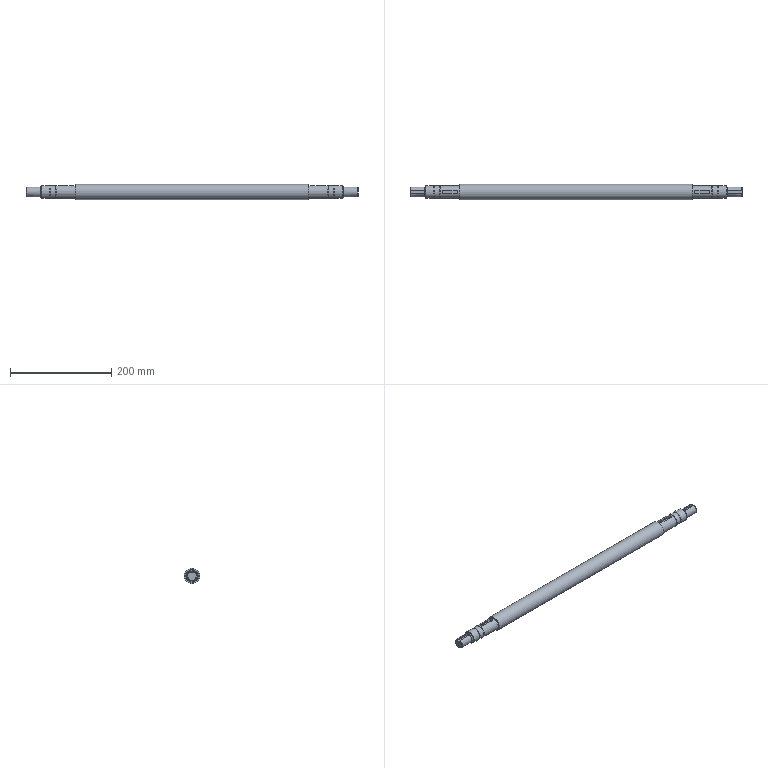NC program | NX | posted with a generic post | part box 656 x 30.5 x 30.5 mm
Lines 1 to 1906 of 2071, first 1725 of 1900 lines:
N10 G17 G21 G94 G90
(ZLEVEL_PROFILE , TOOL : D4)
N12 T04 M6
N14 G54
N16 G17 G0 G90 X-241.716 Y-0.99 S4000 M3
N18 G43 Z30. H4
N20 Z-1.42
N22 G94 G1 X-236.751 Z-1.681 F1000.
N24 X-236.61 Z-1.688
N26 X-236.304 Y-0.895 Z-1.705
N28 X-236.044 Y-0.707 Z-1.722
N30 X-235.856 Y-0.447 Z-1.738
N32 X-235.761 Y-0.141 Z-1.755
N34 Y0.141 Z-1.77
N36 X-235.856 Y0.447 Z-1.787
N38 X-236.044 Y0.707 Z-1.804
N40 X-236.304 Y0.894 Z-1.82
N42 X-236.61 Y0.99 Z-1.837
N44 X-236.776 Z-1.846
N46 X-249.25 Z-2.5
N48 X-261.749 F1400.
N50 G3 X-262.74 Y0. R0.99
N52 X-261.724 Y-0.99 R0.99
N54 G1 X-236.751
N56 G3 X-235.761 Y0. R0.99
N58 X-236.776 Y0.99 R0.99
N60 G1 X-249.25
N62 X-253.792 Z-2.579
N64 X-261.75
N66 G3 X-262.645 Y0.424 R0.99
N68 X-261.724 Y-0.99 R0.99
N70 G1 X-236.75
N72 G3 X-235.855 Y0.424 R0.99
N74 X-236.776 Y0.99 R0.99
N76 G1 X-249.25
N78 X-253.792 Z-2.658
N80 X-261.75
N82 G3 X-262.645 Y0.424 R0.99
N84 X-261.724 Y-0.99 R0.99
N86 G1 X-236.75
N88 G3 X-235.855 Y0.424 R0.99
N90 X-236.776 Y0.99 R0.99
N92 G1 X-249.25
N94 X-253.792 Z-2.737
N96 X-261.75
N98 G3 X-262.645 Y0.424 R0.99
N100 X-261.724 Y-0.99 R0.99
N102 G1 X-236.75
N104 G3 X-235.855 Y0.424 R0.99
N106 X-236.776 Y0.99 R0.99
N108 G1 X-249.25
N110 X-253.792 Z-2.817
N112 X-261.75
N114 G3 X-262.645 Y0.424 R0.99
N116 X-261.723 Y-0.99 R0.99
N118 G1 X-236.75
N120 G3 X-235.855 Y0.424 R0.99
N122 X-236.777 Y0.99 R0.99
N124 G1 X-249.25
N126 X-253.792 Z-2.896
N128 X-261.75
N130 G3 X-262.645 Y0.424 R0.99
N132 X-261.725 Y-0.99 R0.99
N134 G1 X-236.75
N136 G3 X-235.855 Y0.424 R0.99
N138 X-236.775 Y0.99 R0.99
N140 G1 X-249.25
N142 X-253.792 Z-2.975
N144 X-261.75
N146 G3 X-262.645 Y0.424 R0.99
N148 X-261.725 Y-0.99 R0.99
N150 G1 X-236.75
N152 G3 X-235.855 Y0.424 R0.99
N154 X-236.775 Y0.99 R0.99
N156 G1 X-249.25
N158 X-253.792 Z-3.055
N160 X-261.75
N162 G3 X-262.645 Y0.424 R0.99
N164 X-261.725 Y-0.99 R0.99
N166 G1 X-236.75
N168 G3 X-235.855 Y0.424 R0.99
N170 X-236.775 Y0.99 R0.99
N172 G1 X-249.25
N174 X-253.792 Z-3.134
N176 X-261.75
N178 G3 X-262.645 Y0.424 R0.99
N180 X-261.725 Y-0.99 R0.99
N182 G1 X-236.75
N184 G3 X-235.855 Y0.424 R0.99
N186 X-236.775 Y0.99 R0.99
N188 G1 X-249.25
N190 X-253.792 Z-3.213
N192 X-261.75
N194 G3 X-262.645 Y0.424 R0.99
N196 X-261.725 Y-0.99 R0.99
N198 G1 X-236.75
N200 G3 X-235.855 Y0.424 R0.99
N202 X-236.775 Y0.99 R0.99
N204 G1 X-249.25
N206 X-253.792 Z-3.292
N208 X-261.75
N210 G3 X-262.645 Y0.424 R0.99
N212 X-261.725 Y-0.99 R0.99
N214 G1 X-236.75
N216 G3 X-235.855 Y0.424 R0.99
N218 X-236.775 Y0.99 R0.99
N220 G1 X-249.25
N222 X-253.792 Z-3.372
N224 X-261.75
N226 G3 X-262.645 Y0.424 R0.99
N228 X-261.725 Y-0.99 R0.99
N230 G1 X-236.75
N232 G3 X-235.855 Y0.424 R0.99
N234 X-236.775 Y0.99 R0.99
N236 G1 X-249.25
N238 X-253.792 Z-3.451
N240 X-261.75
N242 G3 X-262.645 Y0.424 R0.99
N244 X-261.725 Y-0.99 R0.99
N246 G1 X-236.75
N248 G3 X-235.855 Y0.424 R0.99
N250 X-236.775 Y0.99 R0.99
N252 G1 X-249.25
N254 X-253.792 Z-3.53
N256 X-261.75
N258 G3 X-262.645 Y0.424 R0.99
N260 X-261.725 Y-0.99 R0.99
N262 G1 X-236.75
N264 G3 X-235.855 Y0.424 R0.99
N266 X-236.775 Y0.99 R0.99
N268 G1 X-249.25
N270 X-253.792 Z-3.61
N272 X-261.75
N274 G3 X-262.645 Y0.424 R0.99
N276 X-261.725 Y-0.99 R0.99
N278 G1 X-236.75
N280 G3 X-235.855 Y0.424 R0.99
N282 X-236.775 Y0.99 R0.99
N284 G1 X-249.25
N286 X-253.792 Z-3.689
N288 X-261.75
N290 G3 X-262.645 Y0.424 R0.99
N292 X-261.725 Y-0.99 R0.99
N294 G1 X-236.75
N296 G3 X-235.855 Y0.424 R0.99
N298 X-236.775 Y0.99 R0.99
N300 G1 X-249.25
N302 X-253.792 Z-3.768
N304 X-261.75
N306 G3 X-262.645 Y0.424 R0.99
N308 X-261.725 Y-0.99 R0.99
N310 G1 X-236.75
N312 G3 X-235.855 Y0.424 R0.99
N314 X-236.775 Y0.99 R0.99
N316 G1 X-249.25
N318 X-253.792 Z-3.847
N320 X-261.75
N322 G3 X-262.645 Y0.424 R0.99
N324 X-261.725 Y-0.99 R0.99
N326 G1 X-236.75
N328 G3 X-235.855 Y0.424 R0.99
N330 X-236.775 Y0.99 R0.99
N332 G1 X-249.25
N334 X-253.792 Z-3.927
N336 X-261.75
N338 G3 X-262.645 Y0.424 R0.99
N340 X-261.725 Y-0.99 R0.99
N342 G1 X-236.75
N344 G3 X-235.855 Y0.424 R0.99
N346 X-236.775 Y0.99 R0.99
N348 G1 X-249.25
N350 X-253.792 Z-4.006
N352 X-261.75
N354 G3 X-262.645 Y0.424 R0.99
N356 X-261.725 Y-0.99 R0.99
N358 G1 X-236.75
N360 G3 X-235.855 Y0.424 R0.99
N362 X-236.775 Y0.99 R0.99
N364 G1 X-249.25
N366 X-253.792 Z-4.085
N368 X-261.75
N370 G3 X-262.645 Y0.424 R0.99
N372 X-261.725 Y-0.99 R0.99
N374 G1 X-236.75
N376 G3 X-235.855 Y0.424 R0.99
N378 X-236.775 Y0.99 R0.99
N380 G1 X-249.25
N382 X-253.792 Z-4.164
N384 X-261.75
N386 G3 X-262.645 Y0.424 R0.99
N388 X-261.725 Y-0.99 R0.99
N390 G1 X-236.75
N392 G3 X-235.855 Y0.424 R0.99
N394 X-236.775 Y0.99 R0.99
N396 G1 X-249.25
N398 X-253.792 Z-4.244
N400 X-261.75
N402 G3 X-262.645 Y0.424 R0.99
N404 X-261.725 Y-0.99 R0.99
N406 G1 X-236.75
N408 G3 X-235.855 Y0.424 R0.99
N410 X-236.775 Y0.99 R0.99
N412 G1 X-249.25
N414 X-253.792 Z-4.323
N416 X-261.75
N418 G3 X-262.645 Y0.424 R0.99
N420 X-261.725 Y-0.99 R0.99
N422 G1 X-236.75
N424 G3 X-235.855 Y0.424 R0.99
N426 X-236.775 Y0.99 R0.99
N428 G1 X-249.25
N430 X-253.792 Z-4.402
N432 X-261.75
N434 G3 X-262.645 Y0.424 R0.99
N436 X-261.725 Y-0.99 R0.99
N438 G1 X-236.75
N440 G3 X-235.855 Y0.424 R0.99
N442 X-236.775 Y0.99 R0.99
N444 G1 X-249.25
N446 X-253.792 Z-4.482
N448 X-261.75
N450 G3 X-262.645 Y0.424 R0.99
N452 X-261.725 Y-0.99 R0.99
N454 G1 X-236.75
N456 G3 X-235.855 Y0.424 R0.99
N458 X-236.775 Y0.99 R0.99
N460 G1 X-249.25
N462 X-253.792 Z-4.561
N464 X-261.75
N466 G3 X-262.645 Y0.424 R0.99
N468 X-261.725 Y-0.99 R0.99
N470 G1 X-236.75
N472 G3 X-235.855 Y0.424 R0.99
N474 X-236.775 Y0.99 R0.99
N476 G1 X-249.25
N478 X-253.792 Z-4.64
N480 X-261.75
N482 G3 X-262.645 Y0.424 R0.99
N484 X-261.725 Y-0.99 R0.99
N486 G1 X-236.75
N488 G3 X-235.855 Y0.424 R0.99
N490 X-236.775 Y0.99 R0.99
N492 G1 X-249.25
N494 X-253.792 Z-4.719
N496 X-261.75
N498 G3 X-262.645 Y0.424 R0.99
N500 X-261.725 Y-0.99 R0.99
N502 G1 X-236.75
N504 G3 X-235.855 Y0.424 R0.99
N506 X-236.775 Y0.99 R0.99
N508 G1 X-249.25
N510 X-253.792 Z-4.799
N512 X-261.75
N514 G3 X-262.645 Y0.424 R0.99
N516 X-261.725 Y-0.99 R0.99
N518 G1 X-236.75
N520 G3 X-235.855 Y0.424 R0.99
N522 X-236.775 Y0.99 R0.99
N524 G1 X-249.25
N526 X-253.792 Z-4.878
N528 X-261.75
N530 G3 X-262.645 Y0.424 R0.99
N532 X-261.725 Y-0.99 R0.99
N534 G1 X-236.75
N536 G3 X-235.855 Y0.424 R0.99
N538 X-236.775 Y0.99 R0.99
N540 G1 X-249.25
N542 X-253.792 Z-4.957
N544 X-261.75
N546 G3 X-262.645 Y0.424 R0.99
N548 X-261.725 Y-0.99 R0.99
N550 G1 X-236.75
N552 G3 X-235.855 Y0.424 R0.99
N554 X-236.775 Y0.99 R0.99
N556 G1 X-249.25
N558 X-253.792 Z-5.037
N560 X-261.75
N562 G3 X-262.645 Y0.424 R0.99
N564 X-261.725 Y-0.99 R0.99
N566 G1 X-236.75
N568 G3 X-235.855 Y0.424 R0.99
N570 X-236.775 Y0.99 R0.99
N572 G1 X-249.25
N574 X-253.792 Z-5.116
N576 X-261.75
N578 G3 X-262.645 Y0.424 R0.99
N580 X-261.724 Y-0.99 R0.99
N582 G1 X-236.75
N584 G3 X-235.855 Y0.424 R0.99
N586 X-236.776 Y0.99 R0.99
N588 G1 X-249.25
N590 X-253.792 Z-5.195
N592 X-261.75
N594 G3 X-262.645 Y0.424 R0.99
N596 X-261.724 Y-0.99 R0.99
N598 G1 X-236.75
N600 G3 X-235.855 Y0.424 R0.99
N602 X-236.776 Y0.99 R0.99
N604 G1 X-249.25
N606 X-253.792 Z-5.274
N608 X-261.75
N610 G3 X-262.645 Y0.424 R0.99
N612 X-261.724 Y-0.99 R0.99
N614 G1 X-236.75
N616 G3 X-235.855 Y0.424 R0.99
N618 X-236.776 Y0.99 R0.99
N620 G1 X-249.25
N622 X-253.792 Z-5.354
N624 X-261.75
N626 G3 X-262.645 Y0.424 R0.99
N628 X-261.724 Y-0.99 R0.99
N630 G1 X-236.75
N632 G3 X-235.855 Y0.424 R0.99
N634 X-236.776 Y0.99 R0.99
N636 G1 X-249.25
N638 X-253.792 Z-5.433
N640 X-261.75
N642 G3 X-262.645 Y0.424 R0.99
N644 X-261.724 Y-0.99 R0.99
N646 G1 X-236.75
N648 G3 X-235.855 Y0.424 R0.99
N650 X-236.776 Y0.99 R0.99
N652 G1 X-249.25
N654 X-253.792 Z-5.512
N656 X-261.75
N658 G3 X-262.645 Y0.424 R0.99
N660 X-261.724 Y-0.99 R0.99
N662 G1 X-236.75
N664 G3 X-235.855 Y0.424 R0.99
N666 X-236.776 Y0.99 R0.99
N668 G1 X-249.25
N670 X-253.792 Z-5.591
N672 X-261.75
N674 G3 X-262.645 Y0.424 R0.99
N676 X-261.724 Y-0.99 R0.99
N678 G1 X-236.75
N680 G3 X-235.855 Y0.424 R0.99
N682 X-236.776 Y0.99 R0.99
N684 G1 X-249.25
N686 X-253.792 Z-5.671
N688 X-261.75
N690 G3 X-262.645 Y0.424 R0.99
N692 X-261.724 Y-0.99 R0.99
N694 G1 X-236.75
N696 G3 X-235.855 Y0.424 R0.99
N698 X-236.776 Y0.99 R0.99
N700 G1 X-249.25
N702 X-253.792 Z-5.75
N704 X-261.75
N706 G3 X-262.645 Y0.424 R0.99
N708 X-261.724 Y-0.99 R0.99
N710 G1 X-236.75
N712 G3 X-235.855 Y0.424 R0.99
N714 X-236.776 Y0.99 R0.99
N716 G1 X-253.792
N718 Z-4.75
N720 G0 Z30.
N722 X256.784 Y-0.99
N724 Z-1.42
N726 G1 X261.749 Z-1.681 F1000.
N728 X261.89 Z-1.688
N730 X262.196 Y-0.895 Z-1.705
N732 X262.456 Y-0.707 Z-1.722
N734 X262.644 Y-0.447 Z-1.738
N736 X262.739 Y-0.141 Z-1.755
N738 Y0.141 Z-1.77
N740 X262.644 Y0.447 Z-1.787
N742 X262.456 Y0.707 Z-1.804
N744 X262.196 Y0.894 Z-1.82
N746 X261.89 Y0.99 Z-1.837
N748 X261.724 Z-1.846
N750 X249.25 Z-2.5
N752 X236.751 F1400.
N754 G3 X235.76 Y0. R0.99
N756 X236.776 Y-0.99 R0.99
N758 G1 X261.749
N760 G3 X262.739 Y0. R0.99
N762 X261.724 Y0.99 R0.99
N764 G1 X249.25
N766 X244.708 Z-2.579
N768 X236.75
N770 G3 X235.855 Y0.424 R0.99
N772 X236.776 Y-0.99 R0.99
N774 G1 X261.75
N776 G3 X262.645 Y0.424 R0.99
N778 X261.724 Y0.99 R0.99
N780 G1 X249.25
N782 X244.708 Z-2.658
N784 X236.75
N786 G3 X235.855 Y0.424 R0.99
N788 X236.776 Y-0.99 R0.99
N790 G1 X261.75
N792 G3 X262.645 Y0.424 R0.99
N794 X261.724 Y0.99 R0.99
N796 G1 X249.25
N798 X244.708 Z-2.737
N800 X236.75
N802 G3 X235.855 Y0.424 R0.99
N804 X236.776 Y-0.99 R0.99
N806 G1 X261.75
N808 G3 X262.645 Y0.424 R0.99
N810 X261.724 Y0.99 R0.99
N812 G1 X249.25
N814 X244.708 Z-2.817
N816 X236.75
N818 G3 X235.855 Y0.424 R0.99
N820 X236.777 Y-0.99 R0.99
N822 G1 X261.75
N824 G3 X262.645 Y0.424 R0.99
N826 X261.723 Y0.99 R0.99
N828 G1 X249.25
N830 X244.708 Z-2.896
N832 X236.75
N834 G3 X235.855 Y0.424 R0.99
N836 X236.775 Y-0.99 R0.99
N838 G1 X261.75
N840 G3 X262.645 Y0.424 R0.99
N842 X261.725 Y0.99 R0.99
N844 G1 X249.25
N846 X244.708 Z-2.975
N848 X236.75
N850 G3 X235.855 Y0.424 R0.99
N852 X236.775 Y-0.99 R0.99
N854 G1 X261.75
N856 G3 X262.645 Y0.424 R0.99
N858 X261.725 Y0.99 R0.99
N860 G1 X249.25
N862 X244.708 Z-3.055
N864 X236.75
N866 G3 X235.855 Y0.424 R0.99
N868 X236.775 Y-0.99 R0.99
N870 G1 X261.75
N872 G3 X262.645 Y0.424 R0.99
N874 X261.725 Y0.99 R0.99
N876 G1 X249.25
N878 X244.708 Z-3.134
N880 X236.75
N882 G3 X235.855 Y0.424 R0.99
N884 X236.775 Y-0.99 R0.99
N886 G1 X261.75
N888 G3 X262.645 Y0.424 R0.99
N890 X261.725 Y0.99 R0.99
N892 G1 X249.25
N894 X244.708 Z-3.213
N896 X236.75
N898 G3 X235.855 Y0.424 R0.99
N900 X236.775 Y-0.99 R0.99
N902 G1 X261.75
N904 G3 X262.645 Y0.424 R0.99
N906 X261.725 Y0.99 R0.99
N908 G1 X249.25
N910 X244.708 Z-3.292
N912 X236.75
N914 G3 X235.855 Y0.424 R0.99
N916 X236.775 Y-0.99 R0.99
N918 G1 X261.75
N920 G3 X262.645 Y0.424 R0.99
N922 X261.725 Y0.99 R0.99
N924 G1 X249.25
N926 X244.708 Z-3.372
N928 X236.75
N930 G3 X235.855 Y0.424 R0.99
N932 X236.775 Y-0.99 R0.99
N934 G1 X261.75
N936 G3 X262.645 Y0.424 R0.99
N938 X261.725 Y0.99 R0.99
N940 G1 X249.25
N942 X244.708 Z-3.451
N944 X236.75
N946 G3 X235.855 Y0.424 R0.99
N948 X236.775 Y-0.99 R0.99
N950 G1 X261.75
N952 G3 X262.645 Y0.424 R0.99
N954 X261.725 Y0.99 R0.99
N956 G1 X249.25
N958 X244.708 Z-3.53
N960 X236.75
N962 G3 X235.855 Y0.424 R0.99
N964 X236.775 Y-0.99 R0.99
N966 G1 X261.75
N968 G3 X262.645 Y0.424 R0.99
N970 X261.725 Y0.99 R0.99
N972 G1 X249.25
N974 X244.708 Z-3.61
N976 X236.75
N978 G3 X235.855 Y0.424 R0.99
N980 X236.775 Y-0.99 R0.99
N982 G1 X261.75
N984 G3 X262.645 Y0.424 R0.99
N986 X261.725 Y0.99 R0.99
N988 G1 X249.25
N990 X244.708 Z-3.689
N992 X236.75
N994 G3 X235.855 Y0.424 R0.99
N996 X236.775 Y-0.99 R0.99
N998 G1 X261.75
N1000 G3 X262.645 Y0.424 R0.99
N1002 X261.725 Y0.99 R0.99
N1004 G1 X249.25
N1006 X244.708 Z-3.768
N1008 X236.75
N1010 G3 X235.855 Y0.424 R0.99
N1012 X236.775 Y-0.99 R0.99
N1014 G1 X261.75
N1016 G3 X262.645 Y0.424 R0.99
N1018 X261.725 Y0.99 R0.99
N1020 G1 X249.25
N1022 X244.708 Z-3.847
N1024 X236.75
N1026 G3 X235.855 Y0.424 R0.99
N1028 X236.775 Y-0.99 R0.99
N1030 G1 X261.75
N1032 G3 X262.645 Y0.424 R0.99
N1034 X261.725 Y0.99 R0.99
N1036 G1 X249.25
N1038 X244.708 Z-3.927
N1040 X236.75
N1042 G3 X235.855 Y0.424 R0.99
N1044 X236.775 Y-0.99 R0.99
N1046 G1 X261.75
N1048 G3 X262.645 Y0.424 R0.99
N1050 X261.725 Y0.99 R0.99
N1052 G1 X249.25
N1054 X244.708 Z-4.006
N1056 X236.75
N1058 G3 X235.855 Y0.424 R0.99
N1060 X236.775 Y-0.99 R0.99
N1062 G1 X261.75
N1064 G3 X262.645 Y0.424 R0.99
N1066 X261.725 Y0.99 R0.99
N1068 G1 X249.25
N1070 X244.708 Z-4.085
N1072 X236.75
N1074 G3 X235.855 Y0.424 R0.99
N1076 X236.775 Y-0.99 R0.99
N1078 G1 X261.75
N1080 G3 X262.645 Y0.424 R0.99
N1082 X261.725 Y0.99 R0.99
N1084 G1 X249.25
N1086 X244.708 Z-4.164
N1088 X236.75
N1090 G3 X235.855 Y0.424 R0.99
N1092 X236.775 Y-0.99 R0.99
N1094 G1 X261.75
N1096 G3 X262.645 Y0.424 R0.99
N1098 X261.725 Y0.99 R0.99
N1100 G1 X249.25
N1102 X244.708 Z-4.244
N1104 X236.75
N1106 G3 X235.855 Y0.424 R0.99
N1108 X236.775 Y-0.99 R0.99
N1110 G1 X261.75
N1112 G3 X262.645 Y0.424 R0.99
N1114 X261.725 Y0.99 R0.99
N1116 G1 X249.25
N1118 X244.708 Z-4.323
N1120 X236.75
N1122 G3 X235.855 Y0.424 R0.99
N1124 X236.775 Y-0.99 R0.99
N1126 G1 X261.75
N1128 G3 X262.645 Y0.424 R0.99
N1130 X261.725 Y0.99 R0.99
N1132 G1 X249.25
N1134 X244.708 Z-4.402
N1136 X236.75
N1138 G3 X235.855 Y0.424 R0.99
N1140 X236.775 Y-0.99 R0.99
N1142 G1 X261.75
N1144 G3 X262.645 Y0.424 R0.99
N1146 X261.725 Y0.99 R0.99
N1148 G1 X249.25
N1150 X244.708 Z-4.482
N1152 X236.75
N1154 G3 X235.855 Y0.424 R0.99
N1156 X236.775 Y-0.99 R0.99
N1158 G1 X261.75
N1160 G3 X262.645 Y0.424 R0.99
N1162 X261.725 Y0.99 R0.99
N1164 G1 X249.25
N1166 X244.708 Z-4.561
N1168 X236.75
N1170 G3 X235.855 Y0.424 R0.99
N1172 X236.775 Y-0.99 R0.99
N1174 G1 X261.75
N1176 G3 X262.645 Y0.424 R0.99
N1178 X261.725 Y0.99 R0.99
N1180 G1 X249.25
N1182 X244.708 Z-4.64
N1184 X236.75
N1186 G3 X235.855 Y0.424 R0.99
N1188 X236.775 Y-0.99 R0.99
N1190 G1 X261.75
N1192 G3 X262.645 Y0.424 R0.99
N1194 X261.725 Y0.99 R0.99
N1196 G1 X249.25
N1198 X244.708 Z-4.719
N1200 X236.75
N1202 G3 X235.855 Y0.424 R0.99
N1204 X236.775 Y-0.99 R0.99
N1206 G1 X261.75
N1208 G3 X262.645 Y0.424 R0.99
N1210 X261.725 Y0.99 R0.99
N1212 G1 X249.25
N1214 X244.708 Z-4.799
N1216 X236.75
N1218 G3 X235.855 Y0.424 R0.99
N1220 X236.775 Y-0.99 R0.99
N1222 G1 X261.75
N1224 G3 X262.645 Y0.424 R0.99
N1226 X261.725 Y0.99 R0.99
N1228 G1 X249.25
N1230 X244.708 Z-4.878
N1232 X236.75
N1234 G3 X235.855 Y0.424 R0.99
N1236 X236.775 Y-0.99 R0.99
N1238 G1 X261.75
N1240 G3 X262.645 Y0.424 R0.99
N1242 X261.725 Y0.99 R0.99
N1244 G1 X249.25
N1246 X244.708 Z-4.957
N1248 X236.75
N1250 G3 X235.855 Y0.424 R0.99
N1252 X236.775 Y-0.99 R0.99
N1254 G1 X261.75
N1256 G3 X262.645 Y0.424 R0.99
N1258 X261.725 Y0.99 R0.99
N1260 G1 X249.25
N1262 X244.708 Z-5.037
N1264 X236.75
N1266 G3 X235.855 Y0.424 R0.99
N1268 X236.775 Y-0.99 R0.99
N1270 G1 X261.75
N1272 G3 X262.645 Y0.424 R0.99
N1274 X261.725 Y0.99 R0.99
N1276 G1 X249.25
N1278 X244.708 Z-5.116
N1280 X236.75
N1282 G3 X235.855 Y0.424 R0.99
N1284 X236.776 Y-0.99 R0.99
N1286 G1 X261.75
N1288 G3 X262.645 Y0.424 R0.99
N1290 X261.724 Y0.99 R0.99
N1292 G1 X249.25
N1294 X244.708 Z-5.195
N1296 X236.75
N1298 G3 X235.855 Y0.424 R0.99
N1300 X236.776 Y-0.99 R0.99
N1302 G1 X261.75
N1304 G3 X262.645 Y0.424 R0.99
N1306 X261.724 Y0.99 R0.99
N1308 G1 X249.25
N1310 X244.708 Z-5.274
N1312 X236.75
N1314 G3 X235.855 Y0.424 R0.99
N1316 X236.776 Y-0.99 R0.99
N1318 G1 X261.75
N1320 G3 X262.645 Y0.424 R0.99
N1322 X261.724 Y0.99 R0.99
N1324 G1 X249.25
N1326 X244.708 Z-5.354
N1328 X236.75
N1330 G3 X235.855 Y0.424 R0.99
N1332 X236.776 Y-0.99 R0.99
N1334 G1 X261.75
N1336 G3 X262.645 Y0.424 R0.99
N1338 X261.724 Y0.99 R0.99
N1340 G1 X249.25
N1342 X244.708 Z-5.433
N1344 X236.75
N1346 G3 X235.855 Y0.424 R0.99
N1348 X236.776 Y-0.99 R0.99
N1350 G1 X261.75
N1352 G3 X262.645 Y0.424 R0.99
N1354 X261.724 Y0.99 R0.99
N1356 G1 X249.25
N1358 X244.708 Z-5.512
N1360 X236.75
N1362 G3 X235.855 Y0.424 R0.99
N1364 X236.776 Y-0.99 R0.99
N1366 G1 X261.75
N1368 G3 X262.645 Y0.424 R0.99
N1370 X261.724 Y0.99 R0.99
N1372 G1 X249.25
N1374 X244.708 Z-5.591
N1376 X236.75
N1378 G3 X235.855 Y0.424 R0.99
N1380 X236.776 Y-0.99 R0.99
N1382 G1 X261.75
N1384 G3 X262.645 Y0.424 R0.99
N1386 X261.724 Y0.99 R0.99
N1388 G1 X249.25
N1390 X244.708 Z-5.671
N1392 X236.75
N1394 G3 X235.855 Y0.424 R0.99
N1396 X236.776 Y-0.99 R0.99
N1398 G1 X261.75
N1400 G3 X262.645 Y0.424 R0.99
N1402 X261.724 Y0.99 R0.99
N1404 G1 X249.25
N1406 X244.708 Z-5.75
N1408 X236.75
N1410 G3 X235.855 Y0.424 R0.99
N1412 X236.776 Y-0.99 R0.99
N1414 G1 X261.75
N1416 G3 X262.645 Y0.424 R0.99
N1418 X261.724 Y0.99 R0.99
N1420 G1 X244.708
N1422 Z-4.75
N1424 G0 Z30.
(ZLEVEL_PROFILE_COPY , TOOL : D4)
N1426 X329.958 Y0.299
N1428 Z-5.352
N1430 G1 X329.66 Y0.801 F1000.
N1432 G3 X329.311 Y0.996 R0.4
N1434 G1 X329.053 Y0.993 F1400.
N1436 X328.012
N1438 X328. Y0.99
N1440 X301.935
N1442 X301.788 Y0.96
N1444 G3 X301.018 Y0.112 R0.968
N1446 G1 Y-0.112
N1448 G3 X301.847 Y-0.975 R0.986
N1450 G1 X301.925 Y-0.987
N1452 X301.994 Y-0.99
N1454 X327.98
N1456 X328. Y-0.993
N1458 X329.053
N1460 X329.311 Y-0.996
N1462 G3 X329.66 Y-0.801 R0.4
N1464 G1 X329.957 Y-0.299
N1466 G0 X330.119 Y0.328 Z-5.431
N1468 G1 X329.751 Y0.836 F1000.
N1470 G3 X329.386 Y0.999 R0.4
N1472 G1 X329.335 Y0.994 F1400.
N1474 X328.012 Y0.993
N1476 X328. Y0.99
N1478 X301.935
N1480 X301.788 Y0.96
N1482 G3 X301.018 Y0.112 R0.968
N1484 G1 Y-0.112
N1486 G3 X301.847 Y-0.975 R0.986
N1488 G1 X301.925 Y-0.987
N1490 X301.994 Y-0.99
N1492 X327.98
N1494 X328. Y-0.993
N1496 X329.335 Y-0.994
N1498 X329.386 Y-0.999
N1500 G3 X329.751 Y-0.836 R0.4
N1502 G1 X330.119 Y-0.328
N1504 G0 X330.166 Y0.316 Z-5.51
N1506 G1 X329.82 Y0.828 F1000.
N1508 G3 X329.46 Y1.002 R0.4
N1510 G1 X329.335 Y0.994 F1400.
N1512 X328.012 Y0.992
N1514 X328. Y0.99
N1516 X301.935
N1518 X301.788 Y0.96
N1520 G3 X301.018 Y0.112 R0.968
N1522 G1 Y-0.112
N1524 G3 X301.847 Y-0.975 R0.986
N1526 G1 X301.925 Y-0.987
N1528 X301.994 Y-0.99
N1530 X327.98
N1532 X328. Y-0.992
N1534 X329.335 Y-0.994
N1536 X329.46 Y-1.002
N1538 G3 X329.82 Y-0.828 R0.4
N1540 G1 X330.163 Y-0.32
N1542 G0 X330.209 Y0.305 Z-5.589
N1544 G1 X329.889 Y0.814 F1000.
N1546 G3 X329.535 Y1.001 R0.4
N1548 G1 X329.335 Y0.993 F1400.
N1550 X328.012 Y0.992
N1552 X328. Y0.99
N1554 X301.935
N1556 X301.788 Y0.96
N1558 G3 X301.018 Y0.112 R0.968
N1560 G1 Y-0.112
N1562 G3 X301.847 Y-0.975 R0.986
N1564 G1 X301.925 Y-0.987
N1566 X301.994 Y-0.99
N1568 X327.98
N1570 X328. Y-0.992
N1572 X329.335 Y-0.993
N1574 X329.535 Y-1.001
N1576 G3 X329.889 Y-0.814 R0.4
N1578 G1 X330.206 Y-0.31
N1580 G0 X330.25 Y0.295 Z-5.668
N1582 G1 X329.957 Y0.796 F1000.
N1584 G3 X329.61 Y0.995 R0.4
N1586 G1 X329.335 Y0.993 F1400.
N1588 X328.012 Y0.992
N1590 X328. Y0.99
N1592 X302.
N1594 G3 X301.01 Y0. R0.99
N1596 X302. Y-0.99 R0.99
N1598 G1 X327.98
N1600 X328. Y-0.992
N1602 X329.335 Y-0.993
N1604 X329.61 Y-0.995
N1606 G3 X329.957 Y-0.796 R0.4
N1608 G1 X330.249 Y-0.296
N1610 G0 X330.411 Y0.327 Z-5.747
N1612 G1 X330.048 Y0.835 F1000.
N1614 G3 X329.684 Y1. R0.4
N1616 G1 X329.618 Y0.994 F1400.
N1618 X328.012 Y0.992
N1620 X328. Y0.99
N1622 X302.
N1624 G3 X301.01 Y0. R0.99
N1626 X302. Y-0.99 R0.99
N1628 G1 X327.98
N1630 X328. Y-0.992
N1632 X329.618 Y-0.994
N1634 X329.684 Y-1.
N1636 G3 X330.048 Y-0.835 R0.4
N1638 G1 X330.411 Y-0.327
N1640 G0 X330.458 Y0.314 Z-5.826
N1642 G1 X330.117 Y0.825 F1000.
N1644 G3 X329.759 Y1.003 R0.4
N1646 G1 X329.618 Y0.994 F1400.
N1648 X328.012 Y0.992
N1650 X328. Y0.99
N1652 X302.
N1654 G3 X301.01 Y0. R0.99
N1656 X302. Y-0.99 R0.99
N1658 G1 X327.98
N1660 X328. Y-0.992
N1662 X329.618 Y-0.994
N1664 X329.759 Y-1.003
N1666 G3 X330.117 Y-0.825 R0.4
N1668 G1 X330.455 Y-0.318
N1670 G0 X330.5 Y0.304 Z-5.905
N1672 G1 X330.186 Y0.811 F1000.
N1674 G3 X329.834 Y1. R0.4
N1676 G1 X329.618 Y0.993 F1400.
N1678 X328.012 Y0.992
N1680 X328. Y0.99
N1682 X302.
N1684 G3 X301.01 Y0. R0.99
N1686 X302. Y-0.99 R0.99
N1688 G1 X327.98
N1690 X328. Y-0.992
N1692 X329.618 Y-0.993
N1694 X329.834 Y-1.
N1696 G3 X330.186 Y-0.811 R0.4
N1698 G1 X330.498 Y-0.308
N1700 G0 X330.544 Y0.295 Z-5.984
N1702 G1 X330.255 Y0.795 F1000.
N1704 G3 X329.908 Y0.995 R0.4
N1706 G1 X328.012 Y0.992 F1400.
N1708 X328. Y0.99
N1710 X302.
N1712 G3 X301.01 Y0. R0.99
N1714 X302. Y-0.99 R0.99
N1716 G1 X327.98
N1718 X328. Y-0.992
N1720 X329.908 Y-0.995
N1722 G3 X330.255 Y-0.795 R0.4
N1724 G1 X330.544 Y-0.295
N1726 G0 X330.705 Y0.322 Z-6.063
N1728 G1 X330.345 Y0.833 F1000.
N1730 G3 X329.982 Y1.001 R0.4
N1732 G1 X329.901 Y0.994 F1400.
N1734 X328.012 Y0.992
N1736 X328. Y0.99
N1738 X302.
N1740 G3 X301.01 Y0. R0.99
N1742 X302. Y-0.99 R0.99
N1744 G1 X327.98
N1746 X328. Y-0.992
N1748 X329.901 Y-0.994
N1750 X329.982 Y-1.001
N1752 G3 X330.345 Y-0.833 R0.4
N1754 G1 X330.703 Y-0.325
N1756 G0 X330.747 Y0.316 Z-6.142
N1758 G1 X330.414 Y0.823 F1000.
N1760 G3 X330.057 Y1.002 R0.4
N1762 G1 X329.901 Y0.994 F1400.
N1764 X328.012 Y0.992
N1766 X328. Y0.99
N1768 X302.
N1770 G3 X301.01 Y0. R0.99
N1772 X302. Y-0.99 R0.99
N1774 G1 X327.98
N1776 X328. Y-0.992
N1778 X329.901 Y-0.994
N1780 X330.057 Y-1.002
N1782 G3 X330.414 Y-0.823 R0.4
N1784 G1 X330.747 Y-0.316
N1786 G0 X330.79 Y0.305 Z-6.221
N1788 G1 X330.483 Y0.807 F1000.
N1790 G3 X330.132 Y0.999 R0.4
N1792 G1 X329.901 Y0.993 F1400.
N1794 X328.012 Y0.992
N1796 X328. Y0.99
N1798 X302.
N1800 G3 X301.01 Y0. R0.99
N1802 X302. Y-0.99 R0.99
N1804 G1 X327.98
N1806 X328. Y-0.992
N1808 X329.901 Y-0.993
N1810 X330.132 Y-0.999
N1812 G3 X330.483 Y-0.807 R0.4
N1814 G1 X330.79 Y-0.305
N1816 G0 X330.821 Y0.292 Z-6.3
N1818 G1 X330.53 Y0.794 F1000.
N1820 G3 X330.184 Y0.994 R0.4
N1822 G1 X328.012 Y0.992 F1400.
N1824 X328. Y0.99
N1826 X302.
N1828 G3 X301.01 Y0. R0.99
N1830 X302. Y-0.99 R0.99
N1832 G1 X327.98
N1834 X328. Y-0.992
N1836 X330.184 Y-0.994
N1838 G3 X330.53 Y-0.794 R0.4
N1840 G1 X330.822 Y-0.29
N1842 G0 X330.831 Y0.275 Z-6.379
N1844 G1 X330.531 Y0.794 F1000.
N1846 G3 X330.184 Y0.994 R0.4
N1848 G1 X328.012 Y0.992 F1400.
N1850 X328. Y0.99
N1852 X302.
N1854 G3 X301.01 Y0. R0.99
N1856 X302. Y-0.99 R0.99
N1858 G1 X327.98
N1860 X328. Y-0.992
N1862 X330.184 Y-0.994
N1864 G3 X330.531 Y-0.794 R0.4
N1866 G1 X330.832 Y-0.274
N1868 G0 X330.837 Y0.266 Z-6.458
N1870 G1 X330.531 Y0.794 F1000.
N1872 G3 X330.185 Y0.994 R0.4
N1874 G1 X328.012 Y0.992 F1400.
N1876 X328. Y0.99
N1878 X302.
N1880 G3 X301.01 Y0. R0.99
N1882 X302. Y-0.99 R0.99
N1884 G1 X327.98
N1886 X328. Y-0.992
N1888 X330.185 Y-0.994
N1890 G3 X330.531 Y-0.794 R0.4
N1892 G1 X330.837 Y-0.266
N1894 G0 Y0.266 Z-6.537
N1896 G1 X330.532 Y0.794 F1000.
N1898 G3 X330.185 Y0.993 R0.4
N1900 G1 X328.012 Y0.992 F1400.
N1902 X328. Y0.99
N1904 X302.
N1906 G3 X301.01 Y0. R0.99
N1908 X302. Y-0.99 R0.99
N1910 G1 X327.98
N1912 X328. Y-0.992
N1914 X330.185 Y-0.993
N1916 G3 X330.532 Y-0.794 R0.4
N1918 G1 X330.837 Y-0.266
N1920 G0 Y0.266 Z-6.616
N1922 G1 X330.532 Y0.794 F1000.
N1924 G3 X330.186 Y0.993 R0.4
N1926 G1 X328.012 Y0.992 F1400.
N1928 X328. Y0.99
N1930 X302.
N1932 G3 X301.01 Y0. R0.99
N1934 X302. Y-0.99 R0.99
N1936 G1 X327.98
N1938 X330.186 Y-0.993
N1940 G3 X330.533 Y-0.794 R0.4
N1942 G1 X330.838 Y-0.266
N1944 G0 Y0.266 Z-6.695
N1946 G1 X330.533 Y0.794 F1000.
N1948 G3 X330.186 Y0.993 R0.4
N1950 G1 X328.012 Y0.991 F1400.
N1952 X328. Y0.99
N1954 X302.
N1956 G3 X301.01 Y0. R0.99
N1958 X302. Y-0.99 R0.99
N1960 G1 X327.98
N1962 X330.186 Y-0.993
N1964 G3 X330.533 Y-0.794 R0.4
N1966 G1 X330.839 Y-0.266
N1968 G0 X330.838 Y0.266 Z-6.774
N1970 G1 X330.533 Y0.793 F1000.
N1972 G3 X330.187 Y0.993 R0.4
N1974 G1 X328.012 Y0.991 F1400.
N1976 X328. Y0.99
N1978 X302.
N1980 G3 X301.01 Y0. R0.99
N1982 X302. Y-0.99 R0.99
N1984 G1 X327.98
N1986 X328. Y-0.991
N1988 X330.187 Y-0.993
N1990 G3 X330.533 Y-0.793 R0.4
N1992 G1 X330.838 Y-0.266
N1994 G0 X330.839 Y0.266 Z-6.853
N1996 G1 X330.534 Y0.793 F1000.
N1998 G3 X330.187 Y0.993 R0.4
N2000 G1 X328.012 Y0.991 F1400.
N2002 X328. Y0.99
N2004 X302.
N2006 G3 X301.01 Y0. R0.99
N2008 X302. Y-0.99 R0.99
N2010 G1 X327.98
N2012 X328. Y-0.991
N2014 X330.187 Y-0.993
N2016 G3 X330.534 Y-0.793 R0.4
N2018 G1 X330.839 Y-0.266
N2020 G0 Y0.266 Z-6.932
N2022 G1 X330.534 Y0.793 F1000.
N2024 G3 X330.188 Y0.993 R0.4
N2026 G1 X328.012 Y0.991 F1400.
N2028 X328. Y0.99
N2030 X302.
N2032 G3 X301.01 Y0. R0.99
N2034 X302. Y-0.99 R0.99
N2036 G1 X327.98
N2038 X328. Y-0.991
N2040 X330.188 Y-0.993
N2042 G3 X330.534 Y-0.793 R0.4
N2044 G1 X330.839 Y-0.266
N2046 G0 X330.84 Y0.266 Z-7.011
N2048 G1 X330.535 Y0.793 F1000.
N2050 G3 X330.188 Y0.993 R0.4
N2052 G1 X328.012 Y0.991 F1400.
N2054 X328. Y0.99
N2056 X302.
N2058 G3 X301.01 Y0. R0.99
N2060 X302. Y-0.99 R0.99
N2062 G1 X327.98
N2064 X328. Y-0.991
N2066 X330.188 Y-0.993
N2068 G3 X330.535 Y-0.793 R0.4
N2070 G1 X330.84 Y-0.266
N2072 G0 Y0.266 Z-7.09
N2074 G1 X330.535 Y0.793 F1000.
N2076 G3 X330.189 Y0.993 R0.4
N2078 G1 X328.012 Y0.991 F1400.
N2080 X328. Y0.99
N2082 X302.
N2084 G3 X301.01 Y0. R0.99
N2086 X302. Y-0.99 R0.99
N2088 G1 X327.98
N2090 X328. Y-0.991
N2092 X330.189 Y-0.993
N2094 G3 X330.535 Y-0.793 R0.4
N2096 G1 X330.84 Y-0.266
N2098 G0 Y0.266 Z-7.169
N2100 G1 X330.536 Y0.793 F1000.
N2102 G3 X330.189 Y0.993 R0.4
N2104 G1 X328.012 Y0.991 F1400.
N2106 X328. Y0.99
N2108 X302.
N2110 G3 X301.01 Y0. R0.99
N2112 X302. Y-0.99 R0.99
N2114 G1 X327.98
N2116 X328. Y-0.991
N2118 X330.189 Y-0.993
N2120 G3 X330.536 Y-0.793 R0.4
N2122 G1 X330.841 Y-0.266
N2124 G0 Y0.266 Z-7.248
N2126 G1 X330.536 Y0.793 F1000.
N2128 G3 X330.19 Y0.993 R0.4
N2130 G1 X328. Y0.99 F1400.
N2132 X302.
N2134 G3 X301.01 Y0. R0.99
N2136 X302. Y-0.99 R0.99
N2138 G1 X328. Y-0.991
N2140 X330.19 Y-0.993
N2142 G3 X330.536 Y-0.793 R0.4
N2144 G1 X330.841 Y-0.266
N2146 G0 Y0.266 Z-7.327
N2148 G1 X330.537 Y0.793 F1000.
N2150 G3 X330.19 Y0.992 R0.4
N2152 G1 X328. Y0.99 F1400.
N2154 X302.
N2156 G3 X301.01 Y0. R0.99
N2158 X302. Y-0.99 R0.99
N2160 G1 X328.
N2162 X328.273 Y-1.009
N2164 X328.293 Y-0.991
N2166 X330.19 Y-0.992
N2168 G3 X330.537 Y-0.793 R0.4
N2170 G1 X330.841 Y-0.266
N2172 G0 X330.842 Y0.266 Z-7.406
N2174 G1 X330.537 Y0.793 F1000.
N2176 G3 X330.191 Y0.992 R0.4
N2178 G1 X328. Y0.99 F1400.
N2180 X302.
N2182 G3 X301.01 Y0. R0.99
N2184 X302. Y-0.99 R0.99
N2186 G1 X328.
N2188 X328.273 Y-1.009
N2190 X328.293 Y-0.991
N2192 X330.191 Y-0.992
N2194 G3 X330.538 Y-0.793 R0.4
N2196 G1 X330.842 Y-0.266
N2198 G0 Y0.266 Z-7.485
N2200 G1 X330.538 Y0.793 F1000.
N2202 G3 X330.191 Y0.992 R0.4
N2204 G1 X328. Y0.99 F1400.
N2206 X302.
N2208 G3 X301.01 Y0. R0.99
N2210 X302. Y-0.99 R0.99
N2212 G1 X328.
N2214 X328.273 Y-1.009
N2216 X328.293 Y-0.991
N2218 X330.191 Y-0.992
N2220 G3 X330.538 Y-0.793 R0.4
N2222 G1 X330.842 Y-0.266
N2224 G0 X330.843 Y0.266 Z-7.565
N2226 G1 X330.538 Y0.792 F1000.
N2228 G3 X330.192 Y0.992 R0.4
N2230 G1 X328. Y0.99 F1400.
N2232 X302.
N2234 G3 X301.01 Y0. R0.99
N2236 X302. Y-0.99 R0.99
N2238 G1 X328.
N2240 X328.273 Y-1.009
N2242 X328.293 Y-0.991
N2244 X330.192 Y-0.992
N2246 G3 X330.539 Y-0.792 R0.4
N2248 G1 X330.843 Y-0.266
N2250 G0 Y0.266 Z-7.644
N2252 G1 X330.539 Y0.792 F1000.
N2254 G3 X330.192 Y0.992 R0.4
N2256 G1 X328. Y0.99 F1400.
N2258 X302.
N2260 G3 X301.01 Y0. R0.99
N2262 X302. Y-0.99 R0.99
N2264 G1 X328.
N2266 X328.273 Y-1.009
N2268 X328.293 Y-0.991
N2270 X330.192 Y-0.992
N2272 G3 X330.539 Y-0.792 R0.4
N2274 G1 X330.843 Y-0.266
N2276 G0 Y0.267 Z-7.723
N2278 G1 X330.54 Y0.792 F1000.
N2280 G3 X330.193 Y0.992 R0.4
N2282 G1 X328. Y0.99 F1400.
N2284 X302.
N2286 G3 X301.01 Y0. R0.99
N2288 X302. Y-0.99 R0.99
N2290 G1 X328.
N2292 X328.273 Y-1.009
N2294 X328.293 Y-0.991
N2296 X330.193 Y-0.992
N2298 G3 X330.54 Y-0.792 R0.4
N2300 G1 X330.844 Y-0.266
N2302 G0 Y0.267 Z-7.802
N2304 G1 X330.54 Y0.792 F1000.
N2306 G3 X330.193 Y0.992 R0.4
N2308 G1 X328. Y0.99 F1400.
N2310 X302.
N2312 G3 X301.01 Y0. R0.99
N2314 X302. Y-0.99 R0.99
N2316 G1 X328.
N2318 X328.273 Y-1.009
N2320 X328.293 Y-0.991
N2322 X330.193 Y-0.992
N2324 G3 X330.54 Y-0.792 R0.4
N2326 G1 X330.844 Y-0.266
N2328 G0 Y0.266 Z-7.881
N2330 G1 X330.54 Y0.792 F1000.
N2332 G3 X330.194 Y0.992 R0.4
N2334 G1 X328.084 F1400.
N2336 X328. Y0.99
N2338 X302.
N2340 G3 X301.01 Y0. R0.99
N2342 X302. Y-0.99 R0.99
N2344 G1 X328.
N2346 X328.273 Y-1.009
N2348 X328.293 Y-0.991
N2350 X330.194 Y-0.992
N2352 G3 X330.552 Y-0.814 R0.4
N2354 G1 X330.905 Y-0.281
N2356 G0 X330.906 Y0.282 Z-7.96
N2358 G1 X330.553 Y0.814 F1000.
N2360 G3 X330.194 Y0.992 R0.4
N2362 G1 X328.084 F1400.
N2364 X328. Y0.99
N2366 X302.
N2368 G3 X301.01 Y0. R0.99
N2370 X302. Y-0.99 R0.99
N2372 G1 X328.
N2374 X328.273 Y-1.009
N2376 X328.293 Y-0.99
N2378 X330.194 Y-0.992
N2380 G3 X330.553 Y-0.814 R0.4
N2382 G1 X330.906 Y-0.281
N2384 G0 X330.845 Y0.267 Z-8.039
N2386 G1 X330.542 Y0.792 F1000.
N2388 G3 X330.195 Y0.992 R0.4
N2390 G1 X328. Y0.99 F1400.
N2392 X302.
N2394 G3 X301.01 Y0. R0.99
N2396 X302. Y-0.99 R0.99
N2398 G1 X328.
N2400 X328.273 Y-1.009
N2402 X328.293 Y-0.99
N2404 X330.195 Y-0.992
N2406 G3 X330.553 Y-0.814 R0.4
N2408 G1 X330.906 Y-0.281
N2410 G0 X330.846 Y0.267 Z-8.118
N2412 G1 X330.542 Y0.792 F1000.
N2414 G3 X330.195 Y0.991 R0.4
N2416 G1 X328. Y0.99 F1400.
N2418 X302.
N2420 G3 X301.01 Y0. R0.99
N2422 X302. Y-0.99 R0.99
N2424 G1 X328.
N2426 X328.273 Y-1.009
N2428 X328.293 Y-0.99
N2430 X330.195 Y-0.991
N2432 G3 X330.554 Y-0.813 R0.4
N2434 G1 X330.907 Y-0.281
N2436 G0 X330.846 Y0.267 Z-8.197
N2438 G1 X330.543 Y0.792 F1000.
N2440 G3 X330.196 Y0.991 R0.4
N2442 G1 X328. Y0.99 F1400.
N2444 X302.
N2446 G3 X301.01 Y0. R0.99
N2448 X302. Y-0.99 R0.99
N2450 G1 X328.
N2452 X328.273 Y-1.009
N2454 X328.293 Y-0.99
N2456 X330.196 Y-0.991
N2458 G3 X330.554 Y-0.813 R0.4
N2460 G1 X330.907 Y-0.281
N2462 G0 X330.847 Y0.267 Z-8.276
N2464 G1 X330.543 Y0.792 F1000.
N2466 G3 X330.197 Y0.991 R0.4
N2468 G1 X328. Y0.99 F1400.
N2470 X302.
N2472 G3 X301.01 Y0. R0.99
N2474 X302. Y-0.99 R0.99
N2476 G1 X328.
N2478 X328.273 Y-1.009
N2480 X328.293 Y-0.99
N2482 X330.197 Y-0.991
N2484 G3 X330.555 Y-0.813 R0.4
N2486 G1 X330.908 Y-0.281
N2488 G0 X330.847 Y0.267 Z-8.355
N2490 G1 X330.544 Y0.791 F1000.
N2492 G3 X330.197 Y0.991 R0.4
N2494 G1 X328. Y0.99 F1400.
N2496 X302.
N2498 G3 X301.01 Y0. R0.99
N2500 X302. Y-0.99 R0.99
N2502 G1 X328.
N2504 X328.273 Y-1.009
N2506 X328.293 Y-0.99
N2508 X330.197 Y-0.991
N2510 G3 X330.555 Y-0.813 R0.4
N2512 G1 X330.908 Y-0.281
N2514 G0 X330.847 Y0.267 Z-8.434
N2516 G1 X330.544 Y0.791 F1000.
N2518 G3 X330.198 Y0.991 R0.4
N2520 G1 X328. Y0.99 F1400.
N2522 X302.
N2524 G3 X301.01 Y0. R0.99
N2526 X302. Y-0.99 R0.99
N2528 G1 X328.
N2530 X328.273 Y-1.009
N2532 X328.293 Y-0.99
N2534 X330.198 Y-0.991
N2536 G3 X330.556 Y-0.813 R0.4
N2538 G1 X330.908 Y-0.281
N2540 G0 X330.848 Y0.267 Z-8.513
N2542 G1 X330.545 Y0.791 F1000.
N2544 G3 X330.198 Y0.991 R0.4
N2546 G1 X328. Y0.99 F1400.
N2548 X302.
N2550 G3 X301.01 Y0. R0.99
N2552 X302. Y-0.99 R0.99
N2554 G1 X328.
N2556 X328.273 Y-1.009
N2558 X328.293 Y-0.99
N2560 X330.198 Y-0.991
N2562 G3 X330.556 Y-0.813 R0.4
N2564 G1 X330.909 Y-0.281
N2566 G0 X330.848 Y0.267 Z-8.592
N2568 G1 X330.545 Y0.791 F1000.
N2570 G3 X330.199 Y0.991 R0.4
N2572 G1 X328. Y0.99 F1400.
N2574 X302.
N2576 G3 X301.01 Y0. R0.99
N2578 X302. Y-0.99 R0.99
N2580 G1 X328.
N2582 X328.273 Y-1.009
N2584 X328.293 Y-0.99
N2586 X330.199 Y-0.991
N2588 G3 X330.557 Y-0.813 R0.4
N2590 G1 X330.909 Y-0.281
N2592 G0 X330.849 Y0.267 Z-8.671
N2594 G1 X330.546 Y0.791 F1000.
N2596 G3 X330.199 Y0.991 R0.4
N2598 G1 X328. Y0.99 F1400.
N2600 X302.
N2602 G3 X301.01 Y0. R0.99
N2604 X302. Y-0.99 R0.99
N2606 G1 X328.
N2608 X328.273 Y-1.009
N2610 X328.293 Y-0.99
N2612 X330.199 Y-0.991
N2614 G3 X330.557 Y-0.813 R0.4
N2616 G1 X330.91 Y-0.281
N2618 G0 X330.849 Y0.267 Z-8.75
N2620 G1 X330.546 Y0.791 F1000.
N2622 G3 X330.2 Y0.991 R0.4
N2624 G1 X328. Y0.99 F1400.
N2626 X302.
N2628 G3 X301.01 Y0. R0.99
N2630 X302. Y-0.99 R0.99
N2632 G1 X328.
N2634 X328.273 Y-1.009
N2636 X328.293 Y-0.99
N2638 X330.2 Y-0.991
N2640 G3 X330.558 Y-0.813 R0.4
N2642 G1 X330.91 Y-0.281
N2644 G0 Z30.
N2646 X-329.957 Y-0.299
N2648 Z-5.352
N2650 G1 X-329.66 Y-0.801 F1000.
N2652 G3 X-329.311 Y-0.996 R0.4
N2654 G1 X-329.053 Y-0.993 F1400.
N2656 X-328.
N2658 X-327.904 Y-0.99
N2660 X-301.935
N2662 X-301.836 Y-0.973
N2664 G3 X-301.018 Y-0.112 R0.98
N2666 G1 Y0.112
N2668 G3 X-301.847 Y0.975 R0.986
N2670 G1 X-301.925 Y0.987
N2672 X-301.994 Y0.99
N2674 X-327.904
N2676 X-328. Y0.993
N2678 X-329.053
N2680 X-329.311 Y0.996
N2682 G3 X-329.66 Y0.801 R0.4
N2684 G1 X-329.958 Y0.299
N2686 G0 X-330.119 Y-0.328 Z-5.431
N2688 G1 X-329.751 Y-0.836 F1000.
N2690 G3 X-329.386 Y-0.999 R0.4
N2692 G1 X-329.335 Y-0.994 F1400.
N2694 X-328. Y-0.993
N2696 X-327.904 Y-0.99
N2698 X-301.935
N2700 X-301.836 Y-0.973
N2702 G3 X-301.018 Y-0.112 R0.98
N2704 G1 Y0.112
N2706 G3 X-301.847 Y0.975 R0.986
N2708 G1 X-301.925 Y0.987
N2710 X-301.994 Y0.99
N2712 X-327.904
N2714 X-328. Y0.993
N2716 X-329.335 Y0.994
N2718 X-329.386 Y0.999
N2720 G3 X-329.751 Y0.836 R0.4
N2722 G1 X-330.119 Y0.328
N2724 G0 X-330.165 Y-0.316 Z-5.51
N2726 G1 X-329.82 Y-0.828 F1000.
N2728 G3 X-329.46 Y-1.002 R0.4
N2730 G1 X-329.335 Y-0.994 F1400.
N2732 X-327.922 Y-0.991
N2734 X-327.904 Y-0.99
N2736 X-301.935
N2738 X-301.836 Y-0.973
N2740 G3 X-301.018 Y-0.112 R0.98
N2742 G1 Y0.112
N2744 G3 X-301.847 Y0.975 R0.986
N2746 G1 X-301.925 Y0.987
N2748 X-301.994 Y0.99
N2750 X-327.904
N2752 X-327.922 Y0.991
N2754 X-329.335 Y0.994
N2756 X-329.46 Y1.002
N2758 G3 X-329.82 Y0.828 R0.4
N2760 G1 X-330.163 Y0.32
N2762 G0 X-330.206 Y-0.31 Z-5.589
N2764 G1 X-329.889 Y-0.814 F1000.
N2766 G3 X-329.535 Y-1.001 R0.4
N2768 G1 X-329.335 Y-0.993 F1400.
N2770 X-328. Y-0.992
N2772 X-327.904 Y-0.99
N2774 X-301.935
N2776 X-301.836 Y-0.973
N2778 G3 X-301.018 Y-0.112 R0.98
N2780 G1 Y0.112
N2782 G3 X-301.847 Y0.975 R0.986
N2784 G1 X-301.925 Y0.987
N2786 X-301.994 Y0.99
N2788 X-327.904
N2790 X-328. Y0.992
N2792 X-329.335 Y0.993
N2794 X-329.535 Y1.001
N2796 G3 X-329.889 Y0.814 R0.4
N2798 G1 X-330.206 Y0.31
N2800 G0 X-330.249 Y-0.296 Z-5.668
N2802 G1 X-329.957 Y-0.796 F1000.
N2804 G3 X-329.61 Y-0.995 R0.4
N2806 G1 X-329.335 Y-0.993 F1400.
N2808 X-328. Y-0.992
N2810 X-327.904 Y-0.99
N2812 X-302.
N2814 G3 X-301.01 Y0. R0.99
N2816 X-302. Y0.99 R0.99
N2818 G1 X-327.904
N2820 X-328. Y0.992
N2822 X-329.335 Y0.993
N2824 X-329.61 Y0.995
N2826 G3 X-329.957 Y0.796 R0.4
N2828 G1 X-330.249 Y0.296
N2830 G0 X-330.411 Y-0.327 Z-5.747
N2832 G1 X-330.048 Y-0.835 F1000.
N2834 G3 X-329.684 Y-1. R0.4
N2836 G1 X-329.618 Y-0.994 F1400.
N2838 X-328. Y-0.992
N2840 X-327.904 Y-0.99
N2842 X-302.
N2844 G3 X-301.01 Y0. R0.99
N2846 X-302. Y0.99 R0.99
N2848 G1 X-327.904
N2850 X-328. Y0.992
N2852 X-329.618 Y0.994
N2854 X-329.684 Y1.
N2856 G3 X-330.048 Y0.835 R0.4
N2858 G1 X-330.411 Y0.327
N2860 G0 X-330.458 Y-0.314 Z-5.826
N2862 G1 X-330.117 Y-0.825 F1000.
N2864 G3 X-329.759 Y-1.003 R0.4
N2866 G1 X-329.618 Y-0.994 F1400.
N2868 X-328. Y-0.992
N2870 X-327.904 Y-0.99
N2872 X-302.
N2874 G3 X-301.01 Y0. R0.99
N2876 X-302. Y0.99 R0.99
N2878 G1 X-327.904
N2880 X-328. Y0.992
N2882 X-329.618 Y0.994
N2884 X-329.759 Y1.003
N2886 G3 X-330.117 Y0.825 R0.4
N2888 G1 X-330.455 Y0.318
N2890 G0 X-330.498 Y-0.307 Z-5.905
N2892 G1 X-330.186 Y-0.811 F1000.
N2894 G3 X-329.834 Y-1. R0.4
N2896 G1 X-329.618 Y-0.993 F1400.
N2898 X-328. Y-0.992
N2900 X-327.904 Y-0.99
N2902 X-302.
N2904 G3 X-301.01 Y0. R0.99
N2906 X-302. Y0.99 R0.99
N2908 G1 X-327.904
N2910 X-328. Y0.992
N2912 X-329.618 Y0.993
N2914 X-329.834 Y1.
N2916 G3 X-330.186 Y0.811 R0.4
N2918 G1 X-330.498 Y0.307
N2920 G0 X-330.544 Y-0.295 Z-5.984
N2922 G1 X-330.255 Y-0.795 F1000.
N2924 G3 X-329.908 Y-0.995 R0.4
N2926 G1 X-328. Y-0.992 F1400.
N2928 X-327.904 Y-0.99
N2930 X-302.
N2932 G3 X-301.01 Y0. R0.99
N2934 X-302. Y0.99 R0.99
N2936 G1 X-327.904
N2938 X-328. Y0.992
N2940 X-329.908 Y0.995
N2942 G3 X-330.255 Y0.795 R0.4
N2944 G1 X-330.544 Y0.295
N2946 G0 X-330.703 Y-0.325 Z-6.063
N2948 G1 X-330.345 Y-0.833 F1000.
N2950 G3 X-329.982 Y-1.001 R0.4
N2952 G1 X-329.901 Y-0.994 F1400.
N2954 X-328. Y-0.992
N2956 X-327.904 Y-0.99
N2958 X-302.
N2960 G3 X-301.01 Y0. R0.99
N2962 X-302. Y0.99 R0.99
N2964 G1 X-327.904
N2966 X-328. Y0.992
N2968 X-329.901 Y0.994
N2970 X-329.982 Y1.001
N2972 G3 X-330.345 Y0.833 R0.4
N2974 G1 X-330.703 Y0.325
N2976 G0 X-330.747 Y-0.316 Z-6.142
N2978 G1 X-330.414 Y-0.823 F1000.
N2980 G3 X-330.057 Y-1.002 R0.4
N2982 G1 X-329.901 Y-0.994 F1400.
N2984 X-328. Y-0.992
N2986 X-327.904 Y-0.99
N2988 X-302.
N2990 G3 X-301.01 Y0. R0.99
N2992 X-302. Y0.99 R0.99
N2994 G1 X-327.904
N2996 X-328. Y0.992
N2998 X-329.901 Y0.994
N3000 X-330.057 Y1.002
N3002 G3 X-330.414 Y0.823 R0.4
N3004 G1 X-330.747 Y0.316
N3006 G0 X-330.79 Y-0.305 Z-6.221
N3008 G1 X-330.483 Y-0.807 F1000.
N3010 G3 X-330.132 Y-0.999 R0.4
N3012 G1 X-329.901 Y-0.993 F1400.
N3014 X-328. Y-0.992
N3016 X-327.904 Y-0.99
N3018 X-302.
N3020 G3 X-301.01 Y0. R0.99
N3022 X-302. Y0.99 R0.99
N3024 G1 X-327.904
N3026 X-328. Y0.992
N3028 X-329.901 Y0.993
N3030 X-330.132 Y0.999
N3032 G3 X-330.483 Y0.807 R0.4
N3034 G1 X-330.79 Y0.305
N3036 G0 X-330.822 Y-0.29 Z-6.3
N3038 G1 X-330.53 Y-0.794 F1000.
N3040 G3 X-330.184 Y-0.994 R0.4
N3042 G1 X-328. Y-0.992 F1400.
N3044 X-327.904 Y-0.99
N3046 X-302.
N3048 G3 X-301.01 Y0. R0.99
N3050 X-302. Y0.99 R0.99
N3052 G1 X-327.904
N3054 X-328. Y0.992
N3056 X-330.184 Y0.994
N3058 G3 X-330.53 Y0.794 R0.4
N3060 G1 X-330.822 Y0.289
N3062 G0 X-330.832 Y-0.274 Z-6.379
N3064 G1 X-330.531 Y-0.794 F1000.
N3066 G3 X-330.184 Y-0.994 R0.4
N3068 G1 X-328. Y-0.992 F1400.
N3070 X-327.904 Y-0.99
N3072 X-302.
N3074 G3 X-301.01 Y0. R0.99
N3076 X-302. Y0.99 R0.99
N3078 G1 X-327.904
N3080 X-328. Y0.992
N3082 X-330.184 Y0.994
N3084 G3 X-330.531 Y0.794 R0.4
N3086 G1 X-330.831 Y0.275
N3088 G0 X-330.837 Y-0.266 Z-6.458
N3090 G1 X-330.531 Y-0.794 F1000.
N3092 G3 X-330.185 Y-0.994 R0.4
N3094 G1 X-328. Y-0.992 F1400.
N3096 X-327.904 Y-0.99
N3098 X-302.
N3100 G3 X-301.01 Y0. R0.99
N3102 X-302. Y0.99 R0.99
N3104 G1 X-327.904
N3106 X-328. Y0.992
N3108 X-330.185 Y0.994
N3110 G3 X-330.531 Y0.794 R0.4
N3112 G1 X-330.836 Y0.267
N3114 G0 X-330.837 Y-0.266 Z-6.537
N3116 G1 X-330.532 Y-0.794 F1000.
N3118 G3 X-330.185 Y-0.993 R0.4
N3120 G1 X-328. Y-0.992 F1400.
N3122 X-327.904 Y-0.99
N3124 X-302.
N3126 G3 X-301.01 Y0. R0.99
N3128 X-302. Y0.99 R0.99
N3130 G1 X-327.904
N3132 X-328. Y0.992
N3134 X-330.185 Y0.993
N3136 G3 X-330.532 Y0.794 R0.4
N3138 G1 X-330.837 Y0.267
N3140 G0 Y-0.266 Z-6.616
N3142 G1 X-330.532 Y-0.794 F1000.
N3144 G3 X-330.186 Y-0.993 R0.4
N3146 G1 X-328. Y-0.992 F1400.
N3148 X-327.904 Y-0.99
N3150 X-302.
N3152 G3 X-301.01 Y0. R0.99
N3154 X-302. Y0.99 R0.99
N3156 G1 X-327.904
N3158 X-328. Y0.992
N3160 X-330.186 Y0.993
N3162 G3 X-330.532 Y0.794 R0.4
N3164 G1 X-330.837 Y0.267
N3166 G0 X-330.838 Y-0.266 Z-6.695
N3168 G1 X-330.533 Y-0.794 F1000.
N3170 G3 X-330.186 Y-0.993 R0.4
N3172 G1 X-328. Y-0.991 F1400.
N3174 X-327.904 Y-0.99
N3176 X-302.
N3178 G3 X-301.01 Y0. R0.99
N3180 X-302. Y0.99 R0.99
N3182 G1 X-327.904
N3184 X-328. Y0.991
N3186 X-330.186 Y0.993
N3188 G3 X-330.533 Y0.794 R0.4
N3190 G1 X-330.838 Y0.267
N3192 G0 Y-0.266 Z-6.774
N3194 G1 X-330.533 Y-0.793 F1000.
N3196 G3 X-330.187 Y-0.993 R0.4
N3198 G1 X-328. Y-0.991 F1400.
N3200 X-327.904 Y-0.99
N3202 X-302.
N3204 G3 X-301.01 Y0. R0.99
N3206 X-302. Y0.99 R0.99
N3208 G1 X-327.904
N3210 X-328. Y0.991
N3212 X-330.187 Y0.993
N3214 G3 X-330.533 Y0.793 R0.4
N3216 G1 X-330.838 Y0.267
N3218 G0 X-330.839 Y-0.266 Z-6.853
N3220 G1 X-330.534 Y-0.793 F1000.
N3222 G3 X-330.187 Y-0.993 R0.4
N3224 G1 X-328. Y-0.991 F1400.
N3226 X-327.904 Y-0.99
N3228 X-302.
N3230 G3 X-301.01 Y0. R0.99
N3232 X-302. Y0.99 R0.99
N3234 G1 X-327.904
N3236 X-328. Y0.991
N3238 X-330.187 Y0.993
N3240 G3 X-330.534 Y0.793 R0.4
N3242 G1 X-330.839 Y0.267
N3244 G0 Y-0.266 Z-6.932
N3246 G1 X-330.534 Y-0.793 F1000.
N3248 G3 X-330.188 Y-0.993 R0.4
N3250 G1 X-328. Y-0.991 F1400.
N3252 X-327.904 Y-0.99
N3254 X-302.
N3256 G3 X-301.01 Y0. R0.99
N3258 X-302. Y0.99 R0.99
N3260 G1 X-327.904
N3262 X-328. Y0.991
N3264 X-330.188 Y0.993
N3266 G3 X-330.534 Y0.793 R0.4
N3268 G1 X-330.839 Y0.267
N3270 G0 X-330.84 Y-0.266 Z-7.011
N3272 G1 X-330.535 Y-0.793 F1000.
N3274 G3 X-330.188 Y-0.993 R0.4
N3276 G1 X-328. Y-0.991 F1400.
N3278 X-327.904 Y-0.99
N3280 X-302.
N3282 G3 X-301.01 Y0. R0.99
N3284 X-302. Y0.99 R0.99
N3286 G1 X-327.904
N3288 X-328. Y0.991
N3290 X-330.188 Y0.993
N3292 G3 X-330.535 Y0.793 R0.4
N3294 G1 X-330.839 Y0.267
N3296 G0 X-330.84 Y-0.266 Z-7.09
N3298 G1 X-330.535 Y-0.793 F1000.
N3300 G3 X-330.189 Y-0.993 R0.4
N3302 G1 X-327.904 Y-0.99 F1400.
N3304 X-302.
N3306 G3 X-301.01 Y0. R0.99
N3308 X-302. Y0.99 R0.99
N3310 G1 X-327.904
N3312 X-328. Y0.991
N3314 X-330.189 Y0.993
N3316 G3 X-330.535 Y0.793 R0.4
N3318 G1 X-330.84 Y0.267
N3320 G0 X-330.841 Y-0.266 Z-7.169
N3322 G1 X-330.536 Y-0.793 F1000.
N3324 G3 X-330.189 Y-0.993 R0.4
N3326 G1 X-327.904 Y-0.99 F1400.
N3328 X-302.
N3330 G3 X-301.01 Y0. R0.99
N3332 X-302. Y0.99 R0.99
N3334 G1 X-327.904
N3336 X-330.189 Y0.993
N3338 G3 X-330.536 Y0.793 R0.4
N3340 G1 X-330.841 Y0.267
N3342 G0 Y-0.266 Z-7.248
N3344 G1 X-330.536 Y-0.793 F1000.
N3346 G3 X-330.19 Y-0.993 R0.4
N3348 G1 X-328. Y-0.991 F1400.
N3350 X-327.954 Y-0.99
N3352 X-302.
N3354 G3 X-301.01 Y0. R0.99
N3356 X-302. Y0.99 R0.99
N3358 G1 X-327.954
N3360 X-328. Y0.991
N3362 X-330.19 Y0.993
N3364 G3 X-330.536 Y0.793 R0.4
N3366 G1 X-330.841 Y0.267
N3368 G0 Y-0.266 Z-7.327
N3370 G1 X-330.537 Y-0.793 F1000.
N3372 G3 X-330.19 Y-0.992 R0.4
N3374 G1 X-328. Y-0.991 F1400.
N3376 X-327.922 Y-0.99
N3378 X-302.
N3380 G3 X-301.01 Y0. R0.99
N3382 X-302. Y0.99 R0.99
N3384 G1 X-328.
N3386 X-328.089 Y0.991
N3388 X-330.19 Y0.992
N3390 G3 X-330.537 Y0.793 R0.4
N3392 G1 X-330.841 Y0.267
N3394 G0 X-330.842 Y-0.266 Z-7.406
N3396 G1 X-330.537 Y-0.793 F1000.
N3398 G3 X-330.191 Y-0.992 R0.4
N3400 G1 X-328. Y-0.991 F1400.
N3402 X-327.922 Y-0.99
N3404 X-302.
N3406 G3 X-301.01 Y0. R0.99
N3408 X-302. Y0.99 R0.99
N3410 G1 X-328.
N3412 X-328.089 Y0.991
N3414 X-330.191 Y0.992
N3416 G3 X-330.537 Y0.793 R0.4
N3418 G1 X-330.842 Y0.267
N3420 G0 Y-0.266 Z-7.485
N3422 G1 X-330.538 Y-0.792 F1000.
N3424 G3 X-330.191 Y-0.992 R0.4
N3426 G1 X-328. Y-0.991 F1400.
N3428 X-327.922 Y-0.99
N3430 X-302.
N3432 G3 X-301.01 Y0. R0.99
N3434 X-302. Y0.99 R0.99
N3436 G1 X-328.
N3438 X-328.089 Y0.991
N3440 X-330.191 Y0.992
N3442 G3 X-330.538 Y0.793 R0.4
N3444 G1 X-330.842 Y0.267
N3446 G0 X-330.843 Y-0.266 Z-7.565
N3448 G1 X-330.538 Y-0.792 F1000.
N3450 G3 X-330.192 Y-0.992 R0.4
N3452 G1 X-328. Y-0.991 F1400.
N3454 X-327.922 Y-0.99